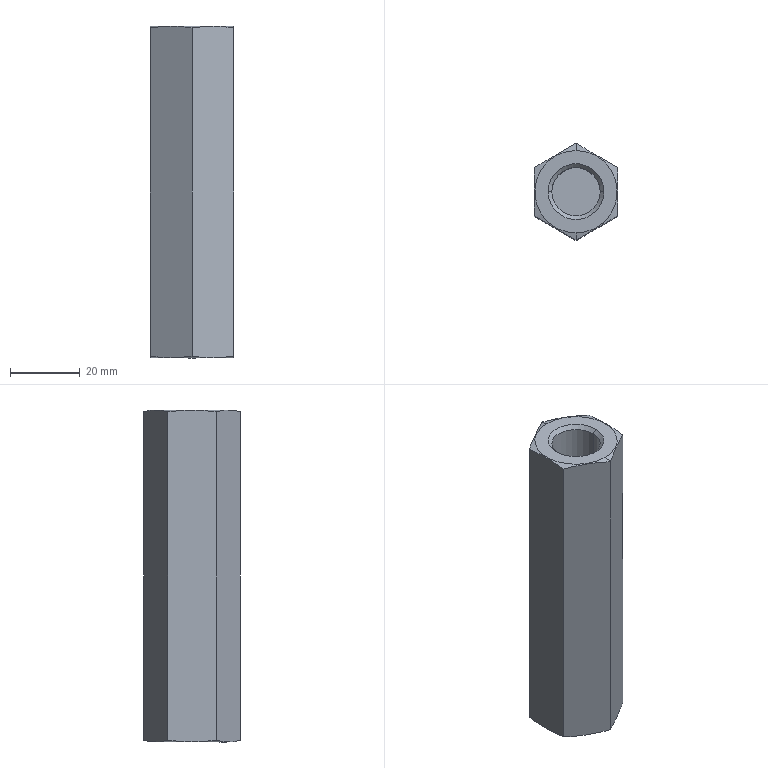Part | SolidWorks | features BaseBody 1 | 1 solid | 22 faces | box 24 x 27.713 x 95 mm | volume 33786 mm3 | plane 10 | cone 8 | cylinder 4 | commonest cylinder face diameters 13.835 x4
STEP:
#1=CARTESIAN_POINT('',(-6.918,0.,-46.418));
#2=VERTEX_POINT('',#1);
#3=CARTESIAN_POINT('',(0.,-6.918,-46.418));
#4=VERTEX_POINT('',#3);
#5=CARTESIAN_POINT('',(0.,0.,-46.418));
#6=DIRECTION('',(0.,0.,1.));
#7=DIRECTION('',(1.,0.,0.));
#8=AXIS2_PLACEMENT_3D('',#5,#6,#7);
#9=CIRCLE('',#8,6.918);
#10=EDGE_CURVE('',#2,#4,#9,.T.);
#11=ORIENTED_EDGE('',*,*,#10,.F.);
#12=CARTESIAN_POINT('',(-6.918,0.,-2.5));
#13=VERTEX_POINT('',#12);
#14=CARTESIAN_POINT('',(-6.918,0.,-47.5));
#15=DIRECTION('',(0.,0.,1.));
#16=VECTOR('',#15,1000.);
#17=LINE('',#14,#16);
#18=EDGE_CURVE('',#2,#13,#17,.T.);
#19=ORIENTED_EDGE('',*,*,#18,.T.);
#20=CARTESIAN_POINT('',(6.918,0.,-2.5));
#21=VERTEX_POINT('',#20);
#22=CARTESIAN_POINT('',(0.,0.,-2.5));
#23=DIRECTION('',(0.,0.,-1.));
#24=DIRECTION('',(1.,0.,0.));
#25=AXIS2_PLACEMENT_3D('',#22,#23,#24);
#26=CIRCLE('',#25,6.918);
#27=EDGE_CURVE('',#21,#13,#26,.T.);
#28=ORIENTED_EDGE('',*,*,#27,.F.);
#29=CARTESIAN_POINT('',(6.918,0.,-46.418));
#30=VERTEX_POINT('',#29);
#31=CARTESIAN_POINT('',(6.918,0.,-47.5));
#32=DIRECTION('',(0.,0.,1.));
#33=VECTOR('',#32,1000.);
#34=LINE('',#31,#33);
#35=EDGE_CURVE('',#30,#21,#34,.T.);
#36=ORIENTED_EDGE('',*,*,#35,.F.);
#37=CARTESIAN_POINT('',(0.,0.,-46.418));
#38=DIRECTION('',(0.,0.,1.));
#39=DIRECTION('',(1.,0.,0.));
#40=AXIS2_PLACEMENT_3D('',#37,#38,#39);
#41=CIRCLE('',#40,6.918);
#42=EDGE_CURVE('',#4,#30,#41,.T.);
#43=ORIENTED_EDGE('',*,*,#42,.F.);
#44=EDGE_LOOP('',(#11,#19,#28,#36,#43));
#45=FACE_OUTER_BOUND('',#44,.T.);
#46=CARTESIAN_POINT('',(0.,0.,-47.5));
#47=DIRECTION('',(0.,0.,1.));
#48=DIRECTION('',(1.,0.,0.));
#49=AXIS2_PLACEMENT_3D('',#46,#47,#48);
#50=CYLINDRICAL_SURFACE('',#49,6.918);
#51=ADVANCED_FACE('',(#45),#50,.F.);
#52=CARTESIAN_POINT('',(0.,6.918,-46.418));
#53=VERTEX_POINT('',#52);
#54=CARTESIAN_POINT('',(0.,0.,-46.418));
#55=DIRECTION('',(0.,0.,1.));
#56=DIRECTION('',(1.,0.,0.));
#57=AXIS2_PLACEMENT_3D('',#54,#55,#56);
#58=CIRCLE('',#57,6.918);
#59=EDGE_CURVE('',#53,#2,#58,.T.);
#60=ORIENTED_EDGE('',*,*,#59,.T.);
#61=ORIENTED_EDGE('',*,*,#10,.T.);
#62=CARTESIAN_POINT('',(0.,-8.,-47.5));
#63=VERTEX_POINT('',#62);
#64=CARTESIAN_POINT('',(0.,-8.,-47.5));
#65=DIRECTION('',(0.,-0.7071,-0.7071));
#66=VECTOR('',#65,1000.);
#67=LINE('',#64,#66);
#68=EDGE_CURVE('',#4,#63,#67,.T.);
#69=ORIENTED_EDGE('',*,*,#68,.T.);
#70=CARTESIAN_POINT('',(0.,8.,-47.5));
#71=VERTEX_POINT('',#70);
#72=CARTESIAN_POINT('',(0.,0.,-47.5));
#73=DIRECTION('',(0.,0.,1.));
#74=DIRECTION('',(0.,1.,0.));
#75=AXIS2_PLACEMENT_3D('',#72,#73,#74);
#76=CIRCLE('',#75,8.);
#77=EDGE_CURVE('',#71,#63,#76,.T.);
#78=ORIENTED_EDGE('',*,*,#77,.F.);
#79=CARTESIAN_POINT('',(0.,8.,-47.5));
#80=DIRECTION('',(0.,0.7071,-0.7071));
#81=VECTOR('',#80,1000.);
#82=LINE('',#79,#81);
#83=EDGE_CURVE('',#53,#71,#82,.T.);
#84=ORIENTED_EDGE('',*,*,#83,.F.);
#85=EDGE_LOOP('',(#60,#61,#69,#78,#84));
#86=FACE_OUTER_BOUND('',#85,.T.);
#87=CARTESIAN_POINT('',(0.,0.,-47.5));
#88=DIRECTION('',(0.,0.,-1.));
#89=DIRECTION('',(0.,1.,0.));
#90=AXIS2_PLACEMENT_3D('',#87,#88,#89);
#91=CONICAL_SURFACE('',#90,8.,0.7854);
#92=ADVANCED_FACE('',(#86),#91,.F.);
#93=CARTESIAN_POINT('',(11.8,0.,-47.5));
#94=VERTEX_POINT('',#93);
#95=CARTESIAN_POINT('',(-11.8,0.,-47.5));
#96=VERTEX_POINT('',#95);
#97=CARTESIAN_POINT('',(0.,0.,-47.5));
#98=DIRECTION('',(0.,0.,1.));
#99=DIRECTION('',(1.,0.,0.));
#100=AXIS2_PLACEMENT_3D('',#97,#98,#99);
#101=CIRCLE('',#100,11.8);
#102=EDGE_CURVE('',#94,#96,#101,.T.);
#103=ORIENTED_EDGE('',*,*,#102,.T.);
#104=CARTESIAN_POINT('',(-12.,0.,-47.446));
#105=VERTEX_POINT('',#104);
#106=CARTESIAN_POINT('',(-13.869,0.,-46.946));
#107=DIRECTION('',(-0.9659,0.,0.2588));
#108=VECTOR('',#107,1000.);
#109=LINE('',#106,#108);
#110=EDGE_CURVE('',#96,#105,#109,.T.);
#111=ORIENTED_EDGE('',*,*,#110,.T.);
#112=CARTESIAN_POINT('',(-12.,6.928,-46.949));
#113=VERTEX_POINT('',#112);
#114=CARTESIAN_POINT('',(-12.,0.,-47.446));
#115=CARTESIAN_POINT('',(-12.,1.155,-47.446));
#116=CARTESIAN_POINT('',(-12.,2.309,-47.401));
#117=CARTESIAN_POINT('',(-12.,4.619,-47.229));
#118=CARTESIAN_POINT('',(-12.,5.774,-47.104));
#119=CARTESIAN_POINT('',(-12.,6.928,-46.949));
#120=B_SPLINE_CURVE_WITH_KNOTS('',3,(#114,#115,#116,#117,#118,#119),.UNSPECIFIED.,.F.,.F.,(4,2,4),(0.006928,0.01039,0.01386),.UNSPECIFIED.);
#121=EDGE_CURVE('',#105,#113,#120,.T.);
#122=ORIENTED_EDGE('',*,*,#121,.T.);
#123=CARTESIAN_POINT('',(-0.000000051,13.856,-46.949));
#124=VERTEX_POINT('',#123);
#125=CARTESIAN_POINT('',(-12.,6.928,-46.949));
#126=CARTESIAN_POINT('',(-11.,7.506,-47.104));
#127=CARTESIAN_POINT('',(-10.,8.083,-47.229));
#128=CARTESIAN_POINT('',(-8.,9.238,-47.401));
#129=CARTESIAN_POINT('',(-6.,10.392,-47.492));
#130=CARTESIAN_POINT('',(-4.,11.547,-47.401));
#131=CARTESIAN_POINT('',(-2.,12.702,-47.229));
#132=CARTESIAN_POINT('',(-1.,13.279,-47.104));
#133=CARTESIAN_POINT('',(-0.000000051,13.856,-46.949));
#134=B_SPLINE_CURVE_WITH_KNOTS('',3,(#125,#126,#127,#128,#129,#130,#131,#132,#133),.UNSPECIFIED.,.F.,.F.,(4,2,1,2,4),(0.,0.003464,0.006928,0.01039,0.01386),.UNSPECIFIED.);
#135=EDGE_CURVE('',#113,#124,#134,.T.);
#136=ORIENTED_EDGE('',*,*,#135,.T.);
#137=CARTESIAN_POINT('',(12.,6.928,-46.949));
#138=VERTEX_POINT('',#137);
#139=CARTESIAN_POINT('',(-0.000000051,13.856,-46.949));
#140=CARTESIAN_POINT('',(1.,13.279,-47.104));
#141=CARTESIAN_POINT('',(2.,12.702,-47.229));
#142=CARTESIAN_POINT('',(4.,11.547,-47.401));
#143=CARTESIAN_POINT('',(6.,10.392,-47.492));
#144=CARTESIAN_POINT('',(8.,9.238,-47.401));
#145=CARTESIAN_POINT('',(10.,8.083,-47.229));
#146=CARTESIAN_POINT('',(11.,7.506,-47.104));
#147=CARTESIAN_POINT('',(12.,6.928,-46.949));
#148=B_SPLINE_CURVE_WITH_KNOTS('',3,(#139,#140,#141,#142,#143,#144,#145,#146,#147),.UNSPECIFIED.,.F.,.F.,(4,2,1,2,4),(0.,0.003464,0.006928,0.01039,0.01386),.UNSPECIFIED.);
#149=EDGE_CURVE('',#124,#138,#148,.T.);
#150=ORIENTED_EDGE('',*,*,#149,.T.);
#151=CARTESIAN_POINT('',(12.,0.,-47.446));
#152=VERTEX_POINT('',#151);
#153=CARTESIAN_POINT('',(12.,6.928,-46.949));
#154=CARTESIAN_POINT('',(12.,5.774,-47.104));
#155=CARTESIAN_POINT('',(12.,4.619,-47.229));
#156=CARTESIAN_POINT('',(12.,2.309,-47.401));
#157=CARTESIAN_POINT('',(12.,1.155,-47.446));
#158=CARTESIAN_POINT('',(12.,0.,-47.446));
#159=B_SPLINE_CURVE_WITH_KNOTS('',3,(#153,#154,#155,#156,#157,#158),.UNSPECIFIED.,.F.,.F.,(4,2,4),(0.,0.003464,0.006928),.UNSPECIFIED.);
#160=EDGE_CURVE('',#138,#152,#159,.T.);
#161=ORIENTED_EDGE('',*,*,#160,.T.);
#162=CARTESIAN_POINT('',(13.869,0.,-46.946));
#163=DIRECTION('',(0.9659,0.,0.2588));
#164=VECTOR('',#163,1000.);
#165=LINE('',#162,#164);
#166=EDGE_CURVE('',#94,#152,#165,.T.);
#167=ORIENTED_EDGE('',*,*,#166,.F.);
#168=EDGE_LOOP('',(#103,#111,#122,#136,#150,#161,#167));
#169=FACE_OUTER_BOUND('',#168,.T.);
#170=CARTESIAN_POINT('',(0.,0.,-46.946));
#171=DIRECTION('',(0.,0.,1.));
#172=DIRECTION('',(1.,0.,0.));
#173=AXIS2_PLACEMENT_3D('',#170,#171,#172);
#174=CONICAL_SURFACE('',#173,13.869,1.309);
#175=ADVANCED_FACE('',(#169),#174,.T.);
#176=CARTESIAN_POINT('',(0.,11.8,47.5));
#177=VERTEX_POINT('',#176);
#178=CARTESIAN_POINT('',(0.,-11.8,47.5));
#179=VERTEX_POINT('',#178);
#180=CARTESIAN_POINT('',(0.,0.,47.5));
#181=DIRECTION('',(0.,0.,-1.));
#182=DIRECTION('',(0.,1.,0.));
#183=AXIS2_PLACEMENT_3D('',#180,#181,#182);
#184=CIRCLE('',#183,11.8);
#185=EDGE_CURVE('',#177,#179,#184,.T.);
#186=ORIENTED_EDGE('',*,*,#185,.T.);
#187=CARTESIAN_POINT('',(0.,-13.856,46.949));
#188=VERTEX_POINT('',#187);
#189=CARTESIAN_POINT('',(0.,-13.869,46.946));
#190=DIRECTION('',(0.,-0.9659,-0.2588));
#191=VECTOR('',#190,1000.);
#192=LINE('',#189,#191);
#193=EDGE_CURVE('',#179,#188,#192,.T.);
#194=ORIENTED_EDGE('',*,*,#193,.T.);
#195=CARTESIAN_POINT('',(12.,-6.928,46.949));
#196=VERTEX_POINT('',#195);
#197=CARTESIAN_POINT('',(0.,-13.856,46.949));
#198=CARTESIAN_POINT('',(1.,-13.279,47.104));
#199=CARTESIAN_POINT('',(2.,-12.702,47.229));
#200=CARTESIAN_POINT('',(4.,-11.547,47.401));
#201=CARTESIAN_POINT('',(6.,-10.392,47.492));
#202=CARTESIAN_POINT('',(8.,-9.238,47.401));
#203=CARTESIAN_POINT('',(10.,-8.083,47.229));
#204=CARTESIAN_POINT('',(11.,-7.506,47.104));
#205=CARTESIAN_POINT('',(12.,-6.928,46.949));
#206=B_SPLINE_CURVE_WITH_KNOTS('',3,(#197,#198,#199,#200,#201,#202,#203,#204,#205),.UNSPECIFIED.,.F.,.F.,(4,2,1,2,4),(0.,0.003464,0.006928,0.01039,0.01386),.UNSPECIFIED.);
#207=EDGE_CURVE('',#188,#196,#206,.T.);
#208=ORIENTED_EDGE('',*,*,#207,.T.);
#209=CARTESIAN_POINT('',(12.,6.928,46.949));
#210=VERTEX_POINT('',#209);
#211=CARTESIAN_POINT('',(12.,-6.928,46.949));
#212=CARTESIAN_POINT('',(12.,-5.774,47.104));
#213=CARTESIAN_POINT('',(12.,-4.619,47.229));
#214=CARTESIAN_POINT('',(12.,-2.309,47.401));
#215=CARTESIAN_POINT('',(12.,0.,47.492));
#216=CARTESIAN_POINT('',(12.,2.309,47.401));
#217=CARTESIAN_POINT('',(12.,4.619,47.229));
#218=CARTESIAN_POINT('',(12.,5.774,47.104));
#219=CARTESIAN_POINT('',(12.,6.928,46.949));
#220=B_SPLINE_CURVE_WITH_KNOTS('',3,(#211,#212,#213,#214,#215,#216,#217,#218,#219),.UNSPECIFIED.,.F.,.F.,(4,2,1,2,4),(0.,0.003464,0.006928,0.01039,0.01386),.UNSPECIFIED.);
#221=EDGE_CURVE('',#196,#210,#220,.T.);
#222=ORIENTED_EDGE('',*,*,#221,.T.);
#223=CARTESIAN_POINT('',(0.,13.856,46.949));
#224=VERTEX_POINT('',#223);
#225=CARTESIAN_POINT('',(12.,6.928,46.949));
#226=CARTESIAN_POINT('',(11.,7.506,47.104));
#227=CARTESIAN_POINT('',(10.,8.083,47.229));
#228=CARTESIAN_POINT('',(8.,9.238,47.401));
#229=CARTESIAN_POINT('',(6.,10.392,47.492));
#230=CARTESIAN_POINT('',(4.,11.547,47.401));
#231=CARTESIAN_POINT('',(2.,12.702,47.229));
#232=CARTESIAN_POINT('',(1.,13.279,47.104));
#233=CARTESIAN_POINT('',(0.,13.856,46.949));
#234=B_SPLINE_CURVE_WITH_KNOTS('',3,(#225,#226,#227,#228,#229,#230,#231,#232,#233),.UNSPECIFIED.,.F.,.F.,(4,2,1,2,4),(0.,0.003464,0.006928,0.01039,0.01386),.UNSPECIFIED.);
#235=EDGE_CURVE('',#210,#224,#234,.T.);
#236=ORIENTED_EDGE('',*,*,#235,.T.);
#237=CARTESIAN_POINT('',(0.,13.869,46.946));
#238=DIRECTION('',(0.,0.9659,-0.2588));
#239=VECTOR('',#238,1000.);
#240=LINE('',#237,#239);
#241=EDGE_CURVE('',#177,#224,#240,.T.);
#242=ORIENTED_EDGE('',*,*,#241,.F.);
#243=EDGE_LOOP('',(#186,#194,#208,#222,#236,#242));
#244=FACE_OUTER_BOUND('',#243,.T.);
#245=CARTESIAN_POINT('',(0.,0.,46.946));
#246=DIRECTION('',(0.,0.,-1.));
#247=DIRECTION('',(0.,1.,0.));
#248=AXIS2_PLACEMENT_3D('',#245,#246,#247);
#249=CONICAL_SURFACE('',#248,13.869,1.309);
#250=ADVANCED_FACE('',(#244),#249,.T.);
#251=CARTESIAN_POINT('',(-6.917,0.,46.417));
#252=VERTEX_POINT('',#251);
#253=CARTESIAN_POINT('',(6.917,0.,46.417));
#254=VERTEX_POINT('',#253);
#255=CARTESIAN_POINT('',(0.,0.,46.417));
#256=DIRECTION('',(0.,0.,1.));
#257=DIRECTION('',(1.,0.,0.));
#258=AXIS2_PLACEMENT_3D('',#255,#256,#257);
#259=CIRCLE('',#258,6.917);
#260=EDGE_CURVE('',#252,#254,#259,.T.);
#261=ORIENTED_EDGE('',*,*,#260,.F.);
#262=CARTESIAN_POINT('',(-8.,0.,47.5));
#263=VERTEX_POINT('',#262);
#264=CARTESIAN_POINT('',(-8.,0.,47.5));
#265=DIRECTION('',(-0.7071,0.,0.7071));
#266=VECTOR('',#265,1000.);
#267=LINE('',#264,#266);
#268=EDGE_CURVE('',#252,#263,#267,.T.);
#269=ORIENTED_EDGE('',*,*,#268,.T.);
#270=CARTESIAN_POINT('',(8.,0.,47.5));
#271=VERTEX_POINT('',#270);
#272=CARTESIAN_POINT('',(0.,0.,47.5));
#273=DIRECTION('',(0.,0.,1.));
#274=DIRECTION('',(1.,0.,0.));
#275=AXIS2_PLACEMENT_3D('',#272,#273,#274);
#276=CIRCLE('',#275,8.);
#277=EDGE_CURVE('',#263,#271,#276,.T.);
#278=ORIENTED_EDGE('',*,*,#277,.T.);
#279=CARTESIAN_POINT('',(8.,0.,47.5));
#280=DIRECTION('',(0.7071,0.,0.7071));
#281=VECTOR('',#280,1000.);
#282=LINE('',#279,#281);
#283=EDGE_CURVE('',#254,#271,#282,.T.);
#284=ORIENTED_EDGE('',*,*,#283,.F.);
#285=EDGE_LOOP('',(#261,#269,#278,#284));
#286=FACE_OUTER_BOUND('',#285,.T.);
#287=CARTESIAN_POINT('',(0.,0.,47.5));
#288=DIRECTION('',(0.,0.,1.));
#289=DIRECTION('',(1.,0.,0.));
#290=AXIS2_PLACEMENT_3D('',#287,#288,#289);
#291=CONICAL_SURFACE('',#290,8.,0.7854);
#292=ADVANCED_FACE('',(#286),#291,.F.);
#293=CARTESIAN_POINT('',(-6.918,0.,2.5));
#294=VERTEX_POINT('',#293);
#295=CARTESIAN_POINT('',(6.918,0.,2.5));
#296=VERTEX_POINT('',#295);
#297=CARTESIAN_POINT('',(0.,0.,2.5));
#298=DIRECTION('',(0.,0.,1.));
#299=DIRECTION('',(1.,0.,0.));
#300=AXIS2_PLACEMENT_3D('',#297,#298,#299);
#301=CIRCLE('',#300,6.918);
#302=EDGE_CURVE('',#294,#296,#301,.T.);
#303=ORIENTED_EDGE('',*,*,#302,.F.);
#304=CARTESIAN_POINT('',(-6.918,0.,-47.5));
#305=DIRECTION('',(0.,0.,1.));
#306=VECTOR('',#305,1000.);
#307=LINE('',#304,#306);
#308=EDGE_CURVE('',#294,#252,#307,.T.);
#309=ORIENTED_EDGE('',*,*,#308,.T.);
#310=ORIENTED_EDGE('',*,*,#260,.T.);
#311=CARTESIAN_POINT('',(6.918,0.,-47.5));
#312=DIRECTION('',(0.,0.,1.));
#313=VECTOR('',#312,1000.);
#314=LINE('',#311,#313);
#315=EDGE_CURVE('',#296,#254,#314,.T.);
#316=ORIENTED_EDGE('',*,*,#315,.F.);
#317=EDGE_LOOP('',(#303,#309,#310,#316));
#318=FACE_OUTER_BOUND('',#317,.T.);
#319=CARTESIAN_POINT('',(0.,0.,-47.5));
#320=DIRECTION('',(0.,0.,1.));
#321=DIRECTION('',(1.,0.,0.));
#322=AXIS2_PLACEMENT_3D('',#319,#320,#321);
#323=CYLINDRICAL_SURFACE('',#322,6.918);
#324=ADVANCED_FACE('',(#318),#323,.F.);
#325=ORIENTED_EDGE('',*,*,#18,.F.);
#326=ORIENTED_EDGE('',*,*,#59,.F.);
#327=CARTESIAN_POINT('',(0.,0.,-46.418));
#328=DIRECTION('',(0.,0.,1.));
#329=DIRECTION('',(1.,0.,0.));
#330=AXIS2_PLACEMENT_3D('',#327,#328,#329);
#331=CIRCLE('',#330,6.918);
#332=EDGE_CURVE('',#30,#53,#331,.T.);
#333=ORIENTED_EDGE('',*,*,#332,.F.);
#334=ORIENTED_EDGE('',*,*,#35,.T.);
#335=CARTESIAN_POINT('',(0.,0.,-2.5));
#336=DIRECTION('',(0.,0.,-1.));
#337=DIRECTION('',(1.,0.,0.));
#338=AXIS2_PLACEMENT_3D('',#335,#336,#337);
#339=CIRCLE('',#338,6.918);
#340=EDGE_CURVE('',#13,#21,#339,.T.);
#341=ORIENTED_EDGE('',*,*,#340,.F.);
#342=EDGE_LOOP('',(#325,#326,#333,#334,#341));
#343=FACE_OUTER_BOUND('',#342,.T.);
#344=CARTESIAN_POINT('',(0.,0.,-47.5));
#345=DIRECTION('',(0.,0.,1.));
#346=DIRECTION('',(1.,0.,0.));
#347=AXIS2_PLACEMENT_3D('',#344,#345,#346);
#348=CYLINDRICAL_SURFACE('',#347,6.918);
#349=ADVANCED_FACE('',(#343),#348,.F.);
#350=ORIENTED_EDGE('',*,*,#68,.F.);
#351=ORIENTED_EDGE('',*,*,#42,.T.);
#352=ORIENTED_EDGE('',*,*,#332,.T.);
#353=ORIENTED_EDGE('',*,*,#83,.T.);
#354=CARTESIAN_POINT('',(0.,0.,-47.5));
#355=DIRECTION('',(0.,0.,1.));
#356=DIRECTION('',(0.,1.,0.));
#357=AXIS2_PLACEMENT_3D('',#354,#355,#356);
#358=CIRCLE('',#357,8.);
#359=EDGE_CURVE('',#63,#71,#358,.T.);
#360=ORIENTED_EDGE('',*,*,#359,.F.);
#361=EDGE_LOOP('',(#350,#351,#352,#353,#360));
#362=FACE_OUTER_BOUND('',#361,.T.);
#363=CARTESIAN_POINT('',(0.,0.,-47.5));
#364=DIRECTION('',(0.,0.,-1.));
#365=DIRECTION('',(0.,1.,0.));
#366=AXIS2_PLACEMENT_3D('',#363,#364,#365);
#367=CONICAL_SURFACE('',#366,8.,0.7854);
#368=ADVANCED_FACE('',(#362),#367,.F.);
#369=ORIENTED_EDGE('',*,*,#27,.T.);
#370=ORIENTED_EDGE('',*,*,#340,.T.);
#371=EDGE_LOOP('',(#369,#370));
#372=FACE_OUTER_BOUND('',#371,.T.);
#373=CARTESIAN_POINT('',(0.,6.918,-2.5));
#374=DIRECTION('',(0.,0.,1.));
#375=DIRECTION('',(1.,0.,0.));
#376=AXIS2_PLACEMENT_3D('',#373,#374,#375);
#377=PLANE('',#376);
#378=ADVANCED_FACE('',(#372),#377,.F.);
#379=ORIENTED_EDGE('',*,*,#102,.F.);
#380=CARTESIAN_POINT('',(0.,0.,-47.5));
#381=DIRECTION('',(0.,0.,1.));
#382=DIRECTION('',(1.,0.,0.));
#383=AXIS2_PLACEMENT_3D('',#380,#381,#382);
#384=CIRCLE('',#383,11.8);
#385=EDGE_CURVE('',#96,#94,#384,.T.);
#386=ORIENTED_EDGE('',*,*,#385,.F.);
#387=EDGE_LOOP('',(#379,#386));
#388=FACE_OUTER_BOUND('',#387,.T.);
#389=ORIENTED_EDGE('',*,*,#77,.T.);
#390=ORIENTED_EDGE('',*,*,#359,.T.);
#391=EDGE_LOOP('',(#389,#390));
#392=FACE_BOUND('',#391,.T.);
#393=CARTESIAN_POINT('',(0.,11.8,-47.5));
#394=DIRECTION('',(0.,0.,1.));
#395=DIRECTION('',(1.,0.,0.));
#396=AXIS2_PLACEMENT_3D('',#393,#394,#395);
#397=PLANE('',#396);
#398=ADVANCED_FACE('',(#388,#392),#397,.F.);
#399=ORIENTED_EDGE('',*,*,#110,.F.);
#400=ORIENTED_EDGE('',*,*,#385,.T.);
#401=ORIENTED_EDGE('',*,*,#166,.T.);
#402=CARTESIAN_POINT('',(12.,-6.928,-46.949));
#403=VERTEX_POINT('',#402);
#404=CARTESIAN_POINT('',(12.,0.,-47.446));
#405=CARTESIAN_POINT('',(12.,-1.155,-47.446));
#406=CARTESIAN_POINT('',(12.,-2.309,-47.401));
#407=CARTESIAN_POINT('',(12.,-4.619,-47.229));
#408=CARTESIAN_POINT('',(12.,-5.774,-47.104));
#409=CARTESIAN_POINT('',(12.,-6.928,-46.949));
#410=B_SPLINE_CURVE_WITH_KNOTS('',3,(#404,#405,#406,#407,#408,#409),.UNSPECIFIED.,.F.,.F.,(4,2,4),(0.006928,0.01039,0.01386),.UNSPECIFIED.);
#411=EDGE_CURVE('',#152,#403,#410,.T.);
#412=ORIENTED_EDGE('',*,*,#411,.T.);
#413=CARTESIAN_POINT('',(0.000000051,-13.856,-46.949));
#414=VERTEX_POINT('',#413);
#415=CARTESIAN_POINT('',(12.,-6.928,-46.949));
#416=CARTESIAN_POINT('',(11.,-7.506,-47.104));
#417=CARTESIAN_POINT('',(10.,-8.083,-47.229));
#418=CARTESIAN_POINT('',(8.,-9.238,-47.401));
#419=CARTESIAN_POINT('',(6.,-10.392,-47.492));
#420=CARTESIAN_POINT('',(4.,-11.547,-47.401));
#421=CARTESIAN_POINT('',(2.,-12.702,-47.229));
#422=CARTESIAN_POINT('',(1.,-13.279,-47.104));
#423=CARTESIAN_POINT('',(0.000000051,-13.856,-46.949));
#424=B_SPLINE_CURVE_WITH_KNOTS('',3,(#415,#416,#417,#418,#419,#420,#421,#422,#423),.UNSPECIFIED.,.F.,.F.,(4,2,1,2,4),(0.,0.003464,0.006928,0.01039,0.01386),.UNSPECIFIED.);
#425=EDGE_CURVE('',#403,#414,#424,.T.);
#426=ORIENTED_EDGE('',*,*,#425,.T.);
#427=CARTESIAN_POINT('',(-12.,-6.928,-46.949));
#428=VERTEX_POINT('',#427);
#429=CARTESIAN_POINT('',(0.000000051,-13.856,-46.949));
#430=CARTESIAN_POINT('',(-1.,-13.279,-47.104));
#431=CARTESIAN_POINT('',(-2.,-12.702,-47.229));
#432=CARTESIAN_POINT('',(-4.,-11.547,-47.401));
#433=CARTESIAN_POINT('',(-6.,-10.392,-47.492));
#434=CARTESIAN_POINT('',(-8.,-9.238,-47.401));
#435=CARTESIAN_POINT('',(-10.,-8.083,-47.229));
#436=CARTESIAN_POINT('',(-11.,-7.506,-47.104));
#437=CARTESIAN_POINT('',(-12.,-6.928,-46.949));
#438=B_SPLINE_CURVE_WITH_KNOTS('',3,(#429,#430,#431,#432,#433,#434,#435,#436,#437),.UNSPECIFIED.,.F.,.F.,(4,2,1,2,4),(0.,0.003464,0.006928,0.01039,0.01386),.UNSPECIFIED.);
#439=EDGE_CURVE('',#414,#428,#438,.T.);
#440=ORIENTED_EDGE('',*,*,#439,.T.);
#441=CARTESIAN_POINT('',(-12.,-6.928,-46.949));
#442=CARTESIAN_POINT('',(-12.,-5.774,-47.104));
#443=CARTESIAN_POINT('',(-12.,-4.619,-47.229));
#444=CARTESIAN_POINT('',(-12.,-2.309,-47.401));
#445=CARTESIAN_POINT('',(-12.,-1.155,-47.446));
#446=CARTESIAN_POINT('',(-12.,0.,-47.446));
#447=B_SPLINE_CURVE_WITH_KNOTS('',3,(#441,#442,#443,#444,#445,#446),.UNSPECIFIED.,.F.,.F.,(4,2,4),(0.,0.003464,0.006928),.UNSPECIFIED.);
#448=EDGE_CURVE('',#428,#105,#447,.T.);
#449=ORIENTED_EDGE('',*,*,#448,.T.);
#450=EDGE_LOOP('',(#399,#400,#401,#412,#426,#440,#449));
#451=FACE_OUTER_BOUND('',#450,.T.);
#452=CARTESIAN_POINT('',(0.,0.,-46.946));
#453=DIRECTION('',(0.,0.,1.));
#454=DIRECTION('',(1.,0.,0.));
#455=AXIS2_PLACEMENT_3D('',#452,#453,#454);
#456=CONICAL_SURFACE('',#455,13.869,1.309);
#457=ADVANCED_FACE('',(#451),#456,.T.);
#458=ORIENTED_EDGE('',*,*,#439,.F.);
#459=CARTESIAN_POINT('',(0.,-13.856,95.));
#460=DIRECTION('',(0.,0.,-1.));
#461=VECTOR('',#460,1000.);
#462=LINE('',#459,#461);
#463=EDGE_CURVE('',#188,#414,#462,.T.);
#464=ORIENTED_EDGE('',*,*,#463,.F.);
#465=CARTESIAN_POINT('',(-12.,-6.928,46.949));
#466=VERTEX_POINT('',#465);
#467=CARTESIAN_POINT('',(-12.,-6.928,46.949));
#468=CARTESIAN_POINT('',(-11.,-7.506,47.104));
#469=CARTESIAN_POINT('',(-10.,-8.083,47.229));
#470=CARTESIAN_POINT('',(-8.,-9.238,47.401));
#471=CARTESIAN_POINT('',(-6.,-10.392,47.492));
#472=CARTESIAN_POINT('',(-4.,-11.547,47.401));
#473=CARTESIAN_POINT('',(-2.,-12.702,47.229));
#474=CARTESIAN_POINT('',(-1.,-13.279,47.104));
#475=CARTESIAN_POINT('',(0.,-13.856,46.949));
#476=B_SPLINE_CURVE_WITH_KNOTS('',3,(#467,#468,#469,#470,#471,#472,#473,#474,#475),.UNSPECIFIED.,.F.,.F.,(4,2,1,2,4),(0.,0.003464,0.006928,0.01039,0.01386),.UNSPECIFIED.);
#477=EDGE_CURVE('',#466,#188,#476,.T.);
#478=ORIENTED_EDGE('',*,*,#477,.F.);
#479=CARTESIAN_POINT('',(-12.,-6.928,95.));
#480=DIRECTION('',(0.,0.,1.));
#481=VECTOR('',#480,1000.);
#482=LINE('',#479,#481);
#483=EDGE_CURVE('',#428,#466,#482,.T.);
#484=ORIENTED_EDGE('',*,*,#483,.F.);
#485=EDGE_LOOP('',(#458,#464,#478,#484));
#486=FACE_OUTER_BOUND('',#485,.T.);
#487=CARTESIAN_POINT('',(-12.,-6.928,95.));
#488=DIRECTION('',(0.5,0.866,0.));
#489=DIRECTION('',(-0.866,0.5,0.));
#490=AXIS2_PLACEMENT_3D('',#487,#488,#489);
#491=PLANE('',#490);
#492=ADVANCED_FACE('',(#486),#491,.F.);
#493=ORIENTED_EDGE('',*,*,#425,.F.);
#494=CARTESIAN_POINT('',(12.,-6.928,95.));
#495=DIRECTION('',(0.,0.,-1.));
#496=VECTOR('',#495,1000.);
#497=LINE('',#494,#496);
#498=EDGE_CURVE('',#196,#403,#497,.T.);
#499=ORIENTED_EDGE('',*,*,#498,.F.);
#500=ORIENTED_EDGE('',*,*,#207,.F.);
#501=ORIENTED_EDGE('',*,*,#463,.T.);
#502=EDGE_LOOP('',(#493,#499,#500,#501));
#503=FACE_OUTER_BOUND('',#502,.T.);
#504=CARTESIAN_POINT('',(0.,-13.856,95.));
#505=DIRECTION('',(-0.5,0.866,0.));
#506=DIRECTION('',(-0.866,-0.5,0.));
#507=AXIS2_PLACEMENT_3D('',#504,#505,#506);
#508=PLANE('',#507);
#509=ADVANCED_FACE('',(#503),#508,.F.);
#510=ORIENTED_EDGE('',*,*,#160,.F.);
#511=CARTESIAN_POINT('',(12.,6.928,95.));
#512=DIRECTION('',(0.,0.,-1.));
#513=VECTOR('',#512,1000.);
#514=LINE('',#511,#513);
#515=EDGE_CURVE('',#210,#138,#514,.T.);
#516=ORIENTED_EDGE('',*,*,#515,.F.);
#517=ORIENTED_EDGE('',*,*,#221,.F.);
#518=ORIENTED_EDGE('',*,*,#498,.T.);
#519=ORIENTED_EDGE('',*,*,#411,.F.);
#520=EDGE_LOOP('',(#510,#516,#517,#518,#519));
#521=FACE_OUTER_BOUND('',#520,.T.);
#522=CARTESIAN_POINT('',(12.,-6.928,95.));
#523=DIRECTION('',(-1.,0.,0.));
#524=DIRECTION('',(0.,0.,1.));
#525=AXIS2_PLACEMENT_3D('',#522,#523,#524);
#526=PLANE('',#525);
#527=ADVANCED_FACE('',(#521),#526,.F.);
#528=ORIENTED_EDGE('',*,*,#149,.F.);
#529=CARTESIAN_POINT('',(0.,13.856,95.));
#530=DIRECTION('',(0.,0.,-1.));
#531=VECTOR('',#530,1000.);
#532=LINE('',#529,#531);
#533=EDGE_CURVE('',#224,#124,#532,.T.);
#534=ORIENTED_EDGE('',*,*,#533,.F.);
#535=ORIENTED_EDGE('',*,*,#235,.F.);
#536=ORIENTED_EDGE('',*,*,#515,.T.);
#537=EDGE_LOOP('',(#528,#534,#535,#536));
#538=FACE_OUTER_BOUND('',#537,.T.);
#539=CARTESIAN_POINT('',(12.,6.928,95.));
#540=DIRECTION('',(-0.5,-0.866,0.));
#541=DIRECTION('',(0.866,-0.5,0.));
#542=AXIS2_PLACEMENT_3D('',#539,#540,#541);
#543=PLANE('',#542);
#544=ADVANCED_FACE('',(#538),#543,.F.);
#545=ORIENTED_EDGE('',*,*,#135,.F.);
#546=CARTESIAN_POINT('',(-12.,6.928,46.949));
#547=VERTEX_POINT('',#546);
#548=CARTESIAN_POINT('',(-12.,6.928,95.));
#549=DIRECTION('',(0.,0.,-1.));
#550=VECTOR('',#549,1000.);
#551=LINE('',#548,#550);
#552=EDGE_CURVE('',#547,#113,#551,.T.);
#553=ORIENTED_EDGE('',*,*,#552,.F.);
#554=CARTESIAN_POINT('',(0.,13.856,46.949));
#555=CARTESIAN_POINT('',(-1.,13.279,47.104));
#556=CARTESIAN_POINT('',(-2.,12.702,47.229));
#557=CARTESIAN_POINT('',(-4.,11.547,47.401));
#558=CARTESIAN_POINT('',(-6.,10.392,47.492));
#559=CARTESIAN_POINT('',(-8.,9.238,47.401));
#560=CARTESIAN_POINT('',(-10.,8.083,47.229));
#561=CARTESIAN_POINT('',(-11.,7.506,47.104));
#562=CARTESIAN_POINT('',(-12.,6.928,46.949));
#563=B_SPLINE_CURVE_WITH_KNOTS('',3,(#554,#555,#556,#557,#558,#559,#560,#561,#562),.UNSPECIFIED.,.F.,.F.,(4,2,1,2,4),(0.,0.003464,0.006928,0.01039,0.01386),.UNSPECIFIED.);
#564=EDGE_CURVE('',#224,#547,#563,.T.);
#565=ORIENTED_EDGE('',*,*,#564,.F.);
#566=ORIENTED_EDGE('',*,*,#533,.T.);
#567=EDGE_LOOP('',(#545,#553,#565,#566));
#568=FACE_OUTER_BOUND('',#567,.T.);
#569=CARTESIAN_POINT('',(0.,13.856,95.));
#570=DIRECTION('',(0.5,-0.866,0.));
#571=DIRECTION('',(0.866,0.5,0.));
#572=AXIS2_PLACEMENT_3D('',#569,#570,#571);
#573=PLANE('',#572);
#574=ADVANCED_FACE('',(#568),#573,.F.);
#575=ORIENTED_EDGE('',*,*,#448,.F.);
#576=ORIENTED_EDGE('',*,*,#483,.T.);
#577=CARTESIAN_POINT('',(-12.,6.928,46.949));
#578=CARTESIAN_POINT('',(-12.,5.774,47.104));
#579=CARTESIAN_POINT('',(-12.,4.619,47.229));
#580=CARTESIAN_POINT('',(-12.,2.309,47.401));
#581=CARTESIAN_POINT('',(-12.,0.,47.492));
#582=CARTESIAN_POINT('',(-12.,-2.309,47.401));
#583=CARTESIAN_POINT('',(-12.,-4.619,47.229));
#584=CARTESIAN_POINT('',(-12.,-5.774,47.104));
#585=CARTESIAN_POINT('',(-12.,-6.928,46.949));
#586=B_SPLINE_CURVE_WITH_KNOTS('',3,(#577,#578,#579,#580,#581,#582,#583,#584,#585),.UNSPECIFIED.,.F.,.F.,(4,2,1,2,4),(0.,0.003464,0.006928,0.01039,0.01386),.UNSPECIFIED.);
#587=EDGE_CURVE('',#547,#466,#586,.T.);
#588=ORIENTED_EDGE('',*,*,#587,.F.);
#589=ORIENTED_EDGE('',*,*,#552,.T.);
#590=ORIENTED_EDGE('',*,*,#121,.F.);
#591=EDGE_LOOP('',(#575,#576,#588,#589,#590));
#592=FACE_OUTER_BOUND('',#591,.T.);
#593=CARTESIAN_POINT('',(-12.,6.928,95.));
#594=DIRECTION('',(1.,0.,0.));
#595=DIRECTION('',(0.,0.,-1.));
#596=AXIS2_PLACEMENT_3D('',#593,#594,#595);
#597=PLANE('',#596);
#598=ADVANCED_FACE('',(#592),#597,.F.);
#599=ORIENTED_EDGE('',*,*,#193,.F.);
#600=CARTESIAN_POINT('',(0.,0.,47.5));
#601=DIRECTION('',(0.,0.,-1.));
#602=DIRECTION('',(0.,1.,0.));
#603=AXIS2_PLACEMENT_3D('',#600,#601,#602);
#604=CIRCLE('',#603,11.8);
#605=EDGE_CURVE('',#179,#177,#604,.T.);
#606=ORIENTED_EDGE('',*,*,#605,.T.);
#607=ORIENTED_EDGE('',*,*,#241,.T.);
#608=ORIENTED_EDGE('',*,*,#564,.T.);
#609=ORIENTED_EDGE('',*,*,#587,.T.);
#610=ORIENTED_EDGE('',*,*,#477,.T.);
#611=EDGE_LOOP('',(#599,#606,#607,#608,#609,#610));
#612=FACE_OUTER_BOUND('',#611,.T.);
#613=CARTESIAN_POINT('',(0.,0.,46.946));
#614=DIRECTION('',(0.,0.,-1.));
#615=DIRECTION('',(0.,1.,0.));
#616=AXIS2_PLACEMENT_3D('',#613,#614,#615);
#617=CONICAL_SURFACE('',#616,13.869,1.309);
#618=ADVANCED_FACE('',(#612),#617,.T.);
#619=CARTESIAN_POINT('',(0.,0.,47.5));
#620=DIRECTION('',(0.,0.,1.));
#621=DIRECTION('',(1.,0.,0.));
#622=AXIS2_PLACEMENT_3D('',#619,#620,#621);
#623=CIRCLE('',#622,8.);
#624=EDGE_CURVE('',#271,#263,#623,.T.);
#625=ORIENTED_EDGE('',*,*,#624,.F.);
#626=ORIENTED_EDGE('',*,*,#277,.F.);
#627=EDGE_LOOP('',(#625,#626));
#628=FACE_BOUND('',#627,.T.);
#629=ORIENTED_EDGE('',*,*,#185,.F.);
#630=ORIENTED_EDGE('',*,*,#605,.F.);
#631=EDGE_LOOP('',(#629,#630));
#632=FACE_OUTER_BOUND('',#631,.T.);
#633=CARTESIAN_POINT('',(0.,8.,47.5));
#634=DIRECTION('',(0.,0.,-1.));
#635=DIRECTION('',(-1.,0.,0.));
#636=AXIS2_PLACEMENT_3D('',#633,#634,#635);
#637=PLANE('',#636);
#638=ADVANCED_FACE('',(#628,#632),#637,.F.);
#639=ORIENTED_EDGE('',*,*,#268,.F.);
#640=CARTESIAN_POINT('',(0.,0.,46.417));
#641=DIRECTION('',(0.,0.,1.));
#642=DIRECTION('',(1.,0.,0.));
#643=AXIS2_PLACEMENT_3D('',#640,#641,#642);
#644=CIRCLE('',#643,6.917);
#645=EDGE_CURVE('',#254,#252,#644,.T.);
#646=ORIENTED_EDGE('',*,*,#645,.F.);
#647=ORIENTED_EDGE('',*,*,#283,.T.);
#648=ORIENTED_EDGE('',*,*,#624,.T.);
#649=EDGE_LOOP('',(#639,#646,#647,#648));
#650=FACE_OUTER_BOUND('',#649,.T.);
#651=CARTESIAN_POINT('',(0.,0.,47.5));
#652=DIRECTION('',(0.,0.,1.));
#653=DIRECTION('',(1.,0.,0.));
#654=AXIS2_PLACEMENT_3D('',#651,#652,#653);
#655=CONICAL_SURFACE('',#654,8.,0.7854);
#656=ADVANCED_FACE('',(#650),#655,.F.);
#657=ORIENTED_EDGE('',*,*,#308,.F.);
#658=CARTESIAN_POINT('',(0.,0.,2.5));
#659=DIRECTION('',(0.,0.,1.));
#660=DIRECTION('',(1.,0.,0.));
#661=AXIS2_PLACEMENT_3D('',#658,#659,#660);
#662=CIRCLE('',#661,6.918);
#663=EDGE_CURVE('',#296,#294,#662,.T.);
#664=ORIENTED_EDGE('',*,*,#663,.F.);
#665=ORIENTED_EDGE('',*,*,#315,.T.);
#666=ORIENTED_EDGE('',*,*,#645,.T.);
#667=EDGE_LOOP('',(#657,#664,#665,#666));
#668=FACE_OUTER_BOUND('',#667,.T.);
#669=CARTESIAN_POINT('',(0.,0.,-47.5));
#670=DIRECTION('',(0.,0.,1.));
#671=DIRECTION('',(1.,0.,0.));
#672=AXIS2_PLACEMENT_3D('',#669,#670,#671);
#673=CYLINDRICAL_SURFACE('',#672,6.918);
#674=ADVANCED_FACE('',(#668),#673,.F.);
#675=ORIENTED_EDGE('',*,*,#663,.T.);
#676=ORIENTED_EDGE('',*,*,#302,.T.);
#677=EDGE_LOOP('',(#675,#676));
#678=FACE_OUTER_BOUND('',#677,.T.);
#679=CARTESIAN_POINT('',(0.,0.,2.5));
#680=DIRECTION('',(0.,0.,-1.));
#681=DIRECTION('',(-1.,0.,0.));
#682=AXIS2_PLACEMENT_3D('',#679,#680,#681);
#683=PLANE('',#682);
#684=ADVANCED_FACE('',(#678),#683,.F.);
#685=CLOSED_SHELL('',(#51,#92,#175,#250,#292,#324,#349,#368,#378,#398,#457,#492,#509,#527,#544,#574,#598,#618,#638,#656,#674,#684));
#686=MANIFOLD_SOLID_BREP('',#685);
#687=CARTESIAN_POINT('',(0.,0.,0.));
#688=DIRECTION('',(0.,0.,1.));
#689=DIRECTION('',(1.,0.,0.));
#690=AXIS2_PLACEMENT_3D('',#687,#688,#689);
#691=(LENGTH_UNIT()NAMED_UNIT(*)SI_UNIT(.MILLI.,.METRE.));
#692=UNCERTAINTY_MEASURE_WITH_UNIT(LENGTH_MEASURE(0.00001),#691,'','');
#693=(NAMED_UNIT(*)PLANE_ANGLE_UNIT()SI_UNIT($,.RADIAN.));
#694=(NAMED_UNIT(*)SI_UNIT($,.STERADIAN.)SOLID_ANGLE_UNIT());
#695=(GEOMETRIC_REPRESENTATION_CONTEXT(3)GLOBAL_UNCERTAINTY_ASSIGNED_CONTEXT((#692))GLOBAL_UNIT_ASSIGNED_CONTEXT((#691,#693,#694))REPRESENTATION_CONTEXT('',''));
#696=ADVANCED_BREP_SHAPE_REPRESENTATION('',(#686,#690),#695);